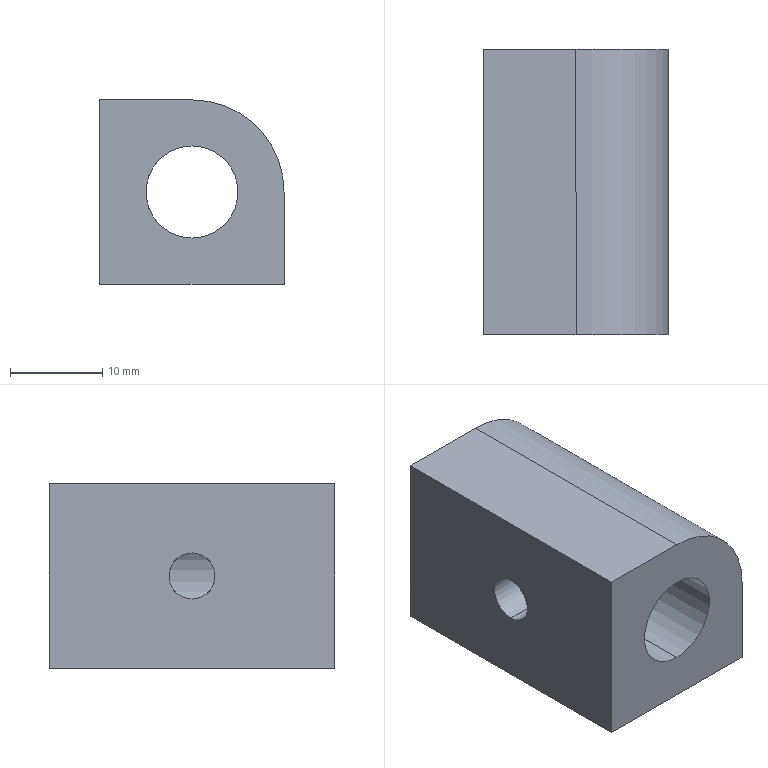Part | STEP file | Sensor mounting block | 1 solid | 27 faces | box 20 x 31 x 20 mm | volume 9027 mm3 | cylinder 13 | cone 8 | plane 6 | commonest cylinder face diameters 2.5 x8 5 x2 10 x2 20 x1